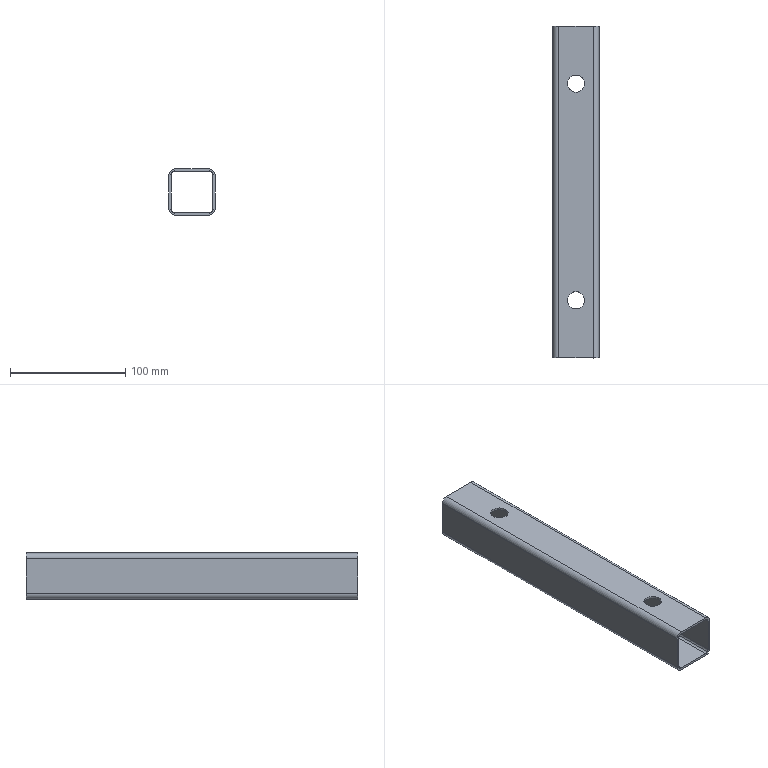Part | NX | features BREP 1 | 1 solid | 44 faces | box 40 x 288 x 40 mm | volume 82180 mm3 | plane 24 | cylinder 20 | commonest cylinder face diameters 6 x8 15 x8 10 x4
STEP:
#1=CARTESIAN_POINT('',(1228.051,-374.5,25.));
#2=VERTEX_POINT('',#1);
#3=CARTESIAN_POINT('',(1228.051,-374.5,27.));
#4=VERTEX_POINT('',#3);
#5=CARTESIAN_POINT('',(1228.051,-374.5,25.));
#6=DIRECTION('',(0.,0.,-1.));
#7=VECTOR('',#6,1000.);
#8=LINE('',#5,#7);
#9=EDGE_CURVE('',#2,#4,#8,.F.);
#10=ORIENTED_EDGE('',*,*,#9,.F.);
#11=CARTESIAN_POINT('',(1213.051,-374.5,25.));
#12=VERTEX_POINT('',#11);
#13=CARTESIAN_POINT('',(1228.051,-374.5,25.));
#14=CARTESIAN_POINT('',(1228.051,-375.305,25.));
#15=CARTESIAN_POINT('',(1227.943,-376.11,25.));
#16=CARTESIAN_POINT('',(1227.727,-376.895,25.));
#17=CARTESIAN_POINT('',(1227.09,-378.389,25.));
#18=CARTESIAN_POINT('',(1226.081,-379.662,25.));
#19=CARTESIAN_POINT('',(1225.494,-380.227,25.));
#20=CARTESIAN_POINT('',(1224.182,-381.185,25.));
#21=CARTESIAN_POINT('',(1222.664,-381.764,25.));
#22=CARTESIAN_POINT('',(1221.871,-381.949,25.));
#23=CARTESIAN_POINT('',(1220.253,-382.102,25.));
#24=CARTESIAN_POINT('',(1218.653,-381.823,25.));
#25=CARTESIAN_POINT('',(1217.876,-381.576,25.));
#26=CARTESIAN_POINT('',(1216.409,-380.881,25.));
#27=CARTESIAN_POINT('',(1215.176,-379.823,25.));
#28=CARTESIAN_POINT('',(1214.634,-379.214,25.));
#29=CARTESIAN_POINT('',(1213.795,-377.964,25.));
#30=CARTESIAN_POINT('',(1213.288,-376.55,25.));
#31=CARTESIAN_POINT('',(1213.13,-375.874,25.));
#32=CARTESIAN_POINT('',(1213.051,-375.187,25.));
#33=CARTESIAN_POINT('',(1213.051,-374.5,25.));
#34=B_SPLINE_CURVE_WITH_KNOTS('',5,(#13,#14,#15,#16,#17,#18,#19,#20,#21,#22,#23,#24,#25,#26,#27,#28,#29,#30,#31,#32,#33),.UNSPECIFIED.,.F.,.F.,(6,3,3,3,3,3,6),(0.,5.692,11.384,17.076,22.768,28.46,33.321),.UNSPECIFIED.);
#35=EDGE_CURVE('',#2,#12,#34,.T.);
#36=ORIENTED_EDGE('',*,*,#35,.T.);
#37=CARTESIAN_POINT('',(1213.051,-374.5,27.));
#38=VERTEX_POINT('',#37);
#39=CARTESIAN_POINT('',(1213.051,-374.5,25.));
#40=DIRECTION('',(0.,0.,-1.));
#41=VECTOR('',#40,1000.);
#42=LINE('',#39,#41);
#43=EDGE_CURVE('',#12,#38,#42,.F.);
#44=ORIENTED_EDGE('',*,*,#43,.T.);
#45=CARTESIAN_POINT('',(1228.051,-374.5,27.));
#46=CARTESIAN_POINT('',(1228.051,-375.305,27.));
#47=CARTESIAN_POINT('',(1227.943,-376.11,27.));
#48=CARTESIAN_POINT('',(1227.727,-376.895,27.));
#49=CARTESIAN_POINT('',(1227.09,-378.389,27.));
#50=CARTESIAN_POINT('',(1226.081,-379.662,27.));
#51=CARTESIAN_POINT('',(1225.494,-380.227,27.));
#52=CARTESIAN_POINT('',(1224.182,-381.185,27.));
#53=CARTESIAN_POINT('',(1222.664,-381.764,27.));
#54=CARTESIAN_POINT('',(1221.871,-381.949,27.));
#55=CARTESIAN_POINT('',(1220.253,-382.102,27.));
#56=CARTESIAN_POINT('',(1218.653,-381.823,27.));
#57=CARTESIAN_POINT('',(1217.876,-381.576,27.));
#58=CARTESIAN_POINT('',(1216.409,-380.881,27.));
#59=CARTESIAN_POINT('',(1215.176,-379.823,27.));
#60=CARTESIAN_POINT('',(1214.634,-379.214,27.));
#61=CARTESIAN_POINT('',(1213.795,-377.964,27.));
#62=CARTESIAN_POINT('',(1213.288,-376.55,27.));
#63=CARTESIAN_POINT('',(1213.13,-375.874,27.));
#64=CARTESIAN_POINT('',(1213.051,-375.187,27.));
#65=CARTESIAN_POINT('',(1213.051,-374.5,27.));
#66=B_SPLINE_CURVE_WITH_KNOTS('',5,(#45,#46,#47,#48,#49,#50,#51,#52,#53,#54,#55,#56,#57,#58,#59,#60,#61,#62,#63,#64,#65),.UNSPECIFIED.,.F.,.F.,(6,3,3,3,3,3,6),(0.,5.692,11.384,17.076,22.768,28.46,33.321),.UNSPECIFIED.);
#67=EDGE_CURVE('',#4,#38,#66,.T.);
#68=ORIENTED_EDGE('',*,*,#67,.F.);
#69=EDGE_LOOP('',(#10,#36,#44,#68));
#70=FACE_BOUND('',#69,.T.);
#71=CARTESIAN_POINT('',(1220.551,-374.5,25.));
#72=DIRECTION('',(0.,0.,-1.));
#73=DIRECTION('',(1.,0.,0.));
#74=AXIS2_PLACEMENT_3D('',#71,#72,#73);
#75=CYLINDRICAL_SURFACE('',#74,7.5);
#76=ADVANCED_FACE('',(#70),#75,.F.);
#77=ORIENTED_EDGE('',*,*,#43,.F.);
#78=CARTESIAN_POINT('',(1213.051,-374.5,25.));
#79=CARTESIAN_POINT('',(1213.051,-373.695,25.));
#80=CARTESIAN_POINT('',(1213.159,-372.89,25.));
#81=CARTESIAN_POINT('',(1213.375,-372.104,25.));
#82=CARTESIAN_POINT('',(1214.013,-370.61,25.));
#83=CARTESIAN_POINT('',(1215.022,-369.337,25.));
#84=CARTESIAN_POINT('',(1215.609,-368.772,25.));
#85=CARTESIAN_POINT('',(1216.921,-367.814,25.));
#86=CARTESIAN_POINT('',(1218.439,-367.235,25.));
#87=CARTESIAN_POINT('',(1219.232,-367.05,25.));
#88=CARTESIAN_POINT('',(1220.849,-366.897,25.));
#89=CARTESIAN_POINT('',(1222.45,-367.176,25.));
#90=CARTESIAN_POINT('',(1223.226,-367.423,25.));
#91=CARTESIAN_POINT('',(1224.694,-368.118,25.));
#92=CARTESIAN_POINT('',(1225.927,-369.176,25.));
#93=CARTESIAN_POINT('',(1226.468,-369.785,25.));
#94=CARTESIAN_POINT('',(1227.308,-371.035,25.));
#95=CARTESIAN_POINT('',(1227.815,-372.449,25.));
#96=CARTESIAN_POINT('',(1227.973,-373.125,25.));
#97=CARTESIAN_POINT('',(1228.051,-373.812,25.));
#98=CARTESIAN_POINT('',(1228.051,-374.5,25.));
#99=B_SPLINE_CURVE_WITH_KNOTS('',5,(#78,#79,#80,#81,#82,#83,#84,#85,#86,#87,#88,#89,#90,#91,#92,#93,#94,#95,#96,#97,#98),.UNSPECIFIED.,.F.,.F.,(6,3,3,3,3,3,6),(0.,5.692,11.384,17.076,22.768,28.46,33.321),.UNSPECIFIED.);
#100=EDGE_CURVE('',#12,#2,#99,.T.);
#101=ORIENTED_EDGE('',*,*,#100,.T.);
#102=ORIENTED_EDGE('',*,*,#9,.T.);
#103=CARTESIAN_POINT('',(1213.051,-374.5,27.));
#104=CARTESIAN_POINT('',(1213.051,-373.695,27.));
#105=CARTESIAN_POINT('',(1213.159,-372.89,27.));
#106=CARTESIAN_POINT('',(1213.375,-372.104,27.));
#107=CARTESIAN_POINT('',(1214.013,-370.61,27.));
#108=CARTESIAN_POINT('',(1215.022,-369.337,27.));
#109=CARTESIAN_POINT('',(1215.609,-368.772,27.));
#110=CARTESIAN_POINT('',(1216.921,-367.814,27.));
#111=CARTESIAN_POINT('',(1218.439,-367.235,27.));
#112=CARTESIAN_POINT('',(1219.232,-367.05,27.));
#113=CARTESIAN_POINT('',(1220.849,-366.897,27.));
#114=CARTESIAN_POINT('',(1222.45,-367.176,27.));
#115=CARTESIAN_POINT('',(1223.226,-367.423,27.));
#116=CARTESIAN_POINT('',(1224.694,-368.118,27.));
#117=CARTESIAN_POINT('',(1225.927,-369.176,27.));
#118=CARTESIAN_POINT('',(1226.468,-369.785,27.));
#119=CARTESIAN_POINT('',(1227.308,-371.035,27.));
#120=CARTESIAN_POINT('',(1227.815,-372.449,27.));
#121=CARTESIAN_POINT('',(1227.973,-373.125,27.));
#122=CARTESIAN_POINT('',(1228.051,-373.812,27.));
#123=CARTESIAN_POINT('',(1228.051,-374.5,27.));
#124=B_SPLINE_CURVE_WITH_KNOTS('',5,(#103,#104,#105,#106,#107,#108,#109,#110,#111,#112,#113,#114,#115,#116,#117,#118,#119,#120,#121,#122,#123),.UNSPECIFIED.,.F.,.F.,(6,3,3,3,3,3,6),(0.,5.692,11.384,17.076,22.768,28.46,33.321),.UNSPECIFIED.);
#125=EDGE_CURVE('',#38,#4,#124,.T.);
#126=ORIENTED_EDGE('',*,*,#125,.F.);
#127=EDGE_LOOP('',(#77,#101,#102,#126));
#128=FACE_BOUND('',#127,.T.);
#129=CARTESIAN_POINT('',(1220.551,-374.5,25.));
#130=DIRECTION('',(0.,0.,-1.));
#131=DIRECTION('',(-1.,0.,0.));
#132=AXIS2_PLACEMENT_3D('',#129,#130,#131);
#133=CYLINDRICAL_SURFACE('',#132,7.5);
#134=ADVANCED_FACE('',(#128),#133,.F.);
#135=CARTESIAN_POINT('',(1213.051,-562.5,25.));
#136=VERTEX_POINT('',#135);
#137=CARTESIAN_POINT('',(1213.051,-562.5,27.));
#138=VERTEX_POINT('',#137);
#139=CARTESIAN_POINT('',(1213.051,-562.5,25.));
#140=DIRECTION('',(0.,0.,1.));
#141=VECTOR('',#140,1000.);
#142=LINE('',#139,#141);
#143=EDGE_CURVE('',#136,#138,#142,.T.);
#144=ORIENTED_EDGE('',*,*,#143,.F.);
#145=CARTESIAN_POINT('',(1228.051,-562.5,25.));
#146=VERTEX_POINT('',#145);
#147=CARTESIAN_POINT('',(1220.551,-562.5,25.));
#148=DIRECTION('',(0.,0.,1.));
#149=DIRECTION('',(1.,0.,0.));
#150=AXIS2_PLACEMENT_3D('',#147,#148,#149);
#151=CIRCLE('',#150,7.5);
#152=EDGE_CURVE('',#146,#136,#151,.T.);
#153=ORIENTED_EDGE('',*,*,#152,.F.);
#154=CARTESIAN_POINT('',(1228.051,-562.5,27.));
#155=VERTEX_POINT('',#154);
#156=CARTESIAN_POINT('',(1228.051,-562.5,25.));
#157=DIRECTION('',(0.,0.,1.));
#158=VECTOR('',#157,1000.);
#159=LINE('',#156,#158);
#160=EDGE_CURVE('',#146,#155,#159,.T.);
#161=ORIENTED_EDGE('',*,*,#160,.T.);
#162=CARTESIAN_POINT('',(1213.051,-562.5,27.));
#163=CARTESIAN_POINT('',(1213.051,-560.53,27.));
#164=CARTESIAN_POINT('',(1214.674,-556.628,27.));
#165=CARTESIAN_POINT('',(1220.551,-554.185,27.));
#166=CARTESIAN_POINT('',(1226.428,-556.628,27.));
#167=CARTESIAN_POINT('',(1228.051,-560.529,27.));
#168=CARTESIAN_POINT('',(1228.051,-562.5,27.));
#169=B_SPLINE_CURVE_WITH_KNOTS('',3,(#162,#163,#164,#165,#166,#167,#168),.UNSPECIFIED.,.F.,.F.,(4,1,1,1,4),(0.,0.25,0.5,0.75,1.),.UNSPECIFIED.);
#170=EDGE_CURVE('',#155,#138,#169,.F.);
#171=ORIENTED_EDGE('',*,*,#170,.T.);
#172=EDGE_LOOP('',(#144,#153,#161,#171));
#173=FACE_BOUND('',#172,.T.);
#174=CARTESIAN_POINT('',(1220.551,-562.5,25.));
#175=DIRECTION('',(0.,0.,1.));
#176=DIRECTION('',(1.,0.,0.));
#177=AXIS2_PLACEMENT_3D('',#174,#175,#176);
#178=CYLINDRICAL_SURFACE('',#177,7.5);
#179=ADVANCED_FACE('',(#173),#178,.F.);
#180=ORIENTED_EDGE('',*,*,#160,.F.);
#181=CARTESIAN_POINT('',(1220.551,-562.5,25.));
#182=DIRECTION('',(0.,0.,1.));
#183=DIRECTION('',(1.,0.,0.));
#184=AXIS2_PLACEMENT_3D('',#181,#182,#183);
#185=CIRCLE('',#184,7.5);
#186=EDGE_CURVE('',#136,#146,#185,.T.);
#187=ORIENTED_EDGE('',*,*,#186,.F.);
#188=ORIENTED_EDGE('',*,*,#143,.T.);
#189=CARTESIAN_POINT('',(1228.051,-562.5,27.));
#190=CARTESIAN_POINT('',(1228.051,-564.469,27.));
#191=CARTESIAN_POINT('',(1226.428,-568.372,27.));
#192=CARTESIAN_POINT('',(1220.551,-570.814,27.));
#193=CARTESIAN_POINT('',(1214.674,-568.371,27.));
#194=CARTESIAN_POINT('',(1213.051,-564.47,27.));
#195=CARTESIAN_POINT('',(1213.051,-562.5,27.));
#196=B_SPLINE_CURVE_WITH_KNOTS('',3,(#189,#190,#191,#192,#193,#194,#195),.UNSPECIFIED.,.F.,.F.,(4,1,1,1,4),(0.,0.25,0.5,0.75,1.),.UNSPECIFIED.);
#197=EDGE_CURVE('',#138,#155,#196,.F.);
#198=ORIENTED_EDGE('',*,*,#197,.T.);
#199=EDGE_LOOP('',(#180,#187,#188,#198));
#200=FACE_BOUND('',#199,.T.);
#201=CARTESIAN_POINT('',(1220.551,-562.5,25.));
#202=DIRECTION('',(0.,0.,1.));
#203=DIRECTION('',(-1.,0.,0.));
#204=AXIS2_PLACEMENT_3D('',#201,#202,#203);
#205=CYLINDRICAL_SURFACE('',#204,7.5);
#206=ADVANCED_FACE('',(#200),#205,.F.);
#207=CARTESIAN_POINT('',(1205.551,-324.5,27.));
#208=VERTEX_POINT('',#207);
#209=CARTESIAN_POINT('',(1205.551,-324.5,25.));
#210=VERTEX_POINT('',#209);
#211=CARTESIAN_POINT('',(1205.551,-324.5,26.));
#212=DIRECTION('',(0.,0.,-1.));
#213=VECTOR('',#212,1000.);
#214=LINE('',#211,#213);
#215=EDGE_CURVE('',#208,#210,#214,.T.);
#216=ORIENTED_EDGE('',*,*,#215,.F.);
#217=CARTESIAN_POINT('',(1235.551,-324.5,27.));
#218=VERTEX_POINT('',#217);
#219=CARTESIAN_POINT('',(1220.551,-324.5,27.));
#220=DIRECTION('',(1.,0.,0.));
#221=VECTOR('',#220,1000.);
#222=LINE('',#219,#221);
#223=EDGE_CURVE('',#208,#218,#222,.T.);
#224=ORIENTED_EDGE('',*,*,#223,.T.);
#225=CARTESIAN_POINT('',(1235.551,-324.5,25.));
#226=VERTEX_POINT('',#225);
#227=CARTESIAN_POINT('',(1235.551,-324.5,26.));
#228=DIRECTION('',(0.,0.,-1.));
#229=VECTOR('',#228,1000.);
#230=LINE('',#227,#229);
#231=EDGE_CURVE('',#218,#226,#230,.T.);
#232=ORIENTED_EDGE('',*,*,#231,.T.);
#233=CARTESIAN_POINT('',(1220.551,-324.5,25.));
#234=DIRECTION('',(1.,0.,0.));
#235=VECTOR('',#234,1000.);
#236=LINE('',#233,#235);
#237=EDGE_CURVE('',#210,#226,#236,.T.);
#238=ORIENTED_EDGE('',*,*,#237,.F.);
#239=EDGE_LOOP('',(#216,#224,#232,#238));
#240=FACE_BOUND('',#239,.T.);
#241=CARTESIAN_POINT('',(1220.551,-324.5,25.));
#242=DIRECTION('',(0.,1.,0.));
#243=DIRECTION('',(1.,0.,0.));
#244=AXIS2_PLACEMENT_3D('',#241,#242,#243);
#245=PLANE('',#244);
#246=ADVANCED_FACE('',(#240),#245,.T.);
#247=CARTESIAN_POINT('',(1240.551,-324.5,30.));
#248=VERTEX_POINT('',#247);
#249=CARTESIAN_POINT('',(1235.551,-324.5,30.));
#250=DIRECTION('',(0.,1.,0.));
#251=DIRECTION('',(1.,0.,0.));
#252=AXIS2_PLACEMENT_3D('',#249,#250,#251);
#253=CIRCLE('',#252,5.);
#254=EDGE_CURVE('',#248,#226,#253,.T.);
#255=ORIENTED_EDGE('',*,*,#254,.T.);
#256=ORIENTED_EDGE('',*,*,#231,.F.);
#257=CARTESIAN_POINT('',(1237.673,-324.5,27.879));
#258=VERTEX_POINT('',#257);
#259=CARTESIAN_POINT('',(1235.551,-324.5,30.));
#260=DIRECTION('',(0.,1.,0.));
#261=DIRECTION('',(1.,0.,0.));
#262=AXIS2_PLACEMENT_3D('',#259,#260,#261);
#263=CIRCLE('',#262,3.);
#264=EDGE_CURVE('',#258,#218,#263,.T.);
#265=ORIENTED_EDGE('',*,*,#264,.F.);
#266=CARTESIAN_POINT('',(1238.551,-324.5,30.));
#267=VERTEX_POINT('',#266);
#268=CARTESIAN_POINT('',(1235.551,-324.5,30.));
#269=DIRECTION('',(0.,1.,0.));
#270=DIRECTION('',(1.,0.,0.));
#271=AXIS2_PLACEMENT_3D('',#268,#269,#270);
#272=CIRCLE('',#271,3.);
#273=EDGE_CURVE('',#267,#258,#272,.T.);
#274=ORIENTED_EDGE('',*,*,#273,.F.);
#275=CARTESIAN_POINT('',(1239.551,-324.5,30.));
#276=DIRECTION('',(1.,0.,0.));
#277=VECTOR('',#276,1000.);
#278=LINE('',#275,#277);
#279=EDGE_CURVE('',#267,#248,#278,.T.);
#280=ORIENTED_EDGE('',*,*,#279,.T.);
#281=EDGE_LOOP('',(#255,#256,#265,#274,#280));
#282=FACE_BOUND('',#281,.T.);
#283=CARTESIAN_POINT('',(1240.551,-324.5,30.));
#284=DIRECTION('',(0.,1.,0.));
#285=DIRECTION('',(-0.3827,0.,-0.9239));
#286=AXIS2_PLACEMENT_3D('',#283,#284,#285);
#287=PLANE('',#286);
#288=ADVANCED_FACE('',(#282),#287,.T.);
#289=ORIENTED_EDGE('',*,*,#67,.T.);
#290=ORIENTED_EDGE('',*,*,#125,.T.);
#291=EDGE_LOOP('',(#289,#290));
#292=FACE_BOUND('',#291,.T.);
#293=ORIENTED_EDGE('',*,*,#170,.F.);
#294=ORIENTED_EDGE('',*,*,#197,.F.);
#295=EDGE_LOOP('',(#293,#294));
#296=FACE_BOUND('',#295,.T.);
#297=CARTESIAN_POINT('',(1205.551,-612.5,27.));
#298=VERTEX_POINT('',#297);
#299=CARTESIAN_POINT('',(1205.551,-468.5,27.));
#300=DIRECTION('',(0.,1.,0.));
#301=VECTOR('',#300,1000.);
#302=LINE('',#299,#301);
#303=EDGE_CURVE('',#298,#208,#302,.T.);
#304=ORIENTED_EDGE('',*,*,#303,.F.);
#305=CARTESIAN_POINT('',(1235.551,-612.5,27.));
#306=VERTEX_POINT('',#305);
#307=CARTESIAN_POINT('',(1220.551,-612.5,27.));
#308=DIRECTION('',(1.,0.,0.));
#309=VECTOR('',#308,1000.);
#310=LINE('',#307,#309);
#311=EDGE_CURVE('',#298,#306,#310,.T.);
#312=ORIENTED_EDGE('',*,*,#311,.T.);
#313=CARTESIAN_POINT('',(1235.551,-468.5,27.));
#314=DIRECTION('',(0.,1.,0.));
#315=VECTOR('',#314,1000.);
#316=LINE('',#313,#315);
#317=EDGE_CURVE('',#306,#218,#316,.T.);
#318=ORIENTED_EDGE('',*,*,#317,.T.);
#319=ORIENTED_EDGE('',*,*,#223,.F.);
#320=EDGE_LOOP('',(#304,#312,#318,#319));
#321=FACE_BOUND('',#320,.T.);
#322=CARTESIAN_POINT('',(1200.551,-612.5,27.));
#323=DIRECTION('',(0.,0.,1.));
#324=DIRECTION('',(1.,0.,0.));
#325=AXIS2_PLACEMENT_3D('',#322,#323,#324);
#326=PLANE('',#325);
#327=ADVANCED_FACE('',(#292,#296,#321),#326,.T.);
#328=ORIENTED_EDGE('',*,*,#100,.F.);
#329=ORIENTED_EDGE('',*,*,#35,.F.);
#330=EDGE_LOOP('',(#328,#329));
#331=FACE_BOUND('',#330,.T.);
#332=ORIENTED_EDGE('',*,*,#186,.T.);
#333=ORIENTED_EDGE('',*,*,#152,.T.);
#334=EDGE_LOOP('',(#332,#333));
#335=FACE_BOUND('',#334,.T.);
#336=ORIENTED_EDGE('',*,*,#237,.T.);
#337=CARTESIAN_POINT('',(1235.551,-612.5,25.));
#338=VERTEX_POINT('',#337);
#339=CARTESIAN_POINT('',(1235.551,-468.5,25.));
#340=DIRECTION('',(0.,1.,0.));
#341=VECTOR('',#340,1000.);
#342=LINE('',#339,#341);
#343=EDGE_CURVE('',#338,#226,#342,.T.);
#344=ORIENTED_EDGE('',*,*,#343,.F.);
#345=CARTESIAN_POINT('',(1205.551,-612.5,25.));
#346=VERTEX_POINT('',#345);
#347=CARTESIAN_POINT('',(1220.551,-612.5,25.));
#348=DIRECTION('',(1.,0.,0.));
#349=VECTOR('',#348,1000.);
#350=LINE('',#347,#349);
#351=EDGE_CURVE('',#346,#338,#350,.T.);
#352=ORIENTED_EDGE('',*,*,#351,.F.);
#353=CARTESIAN_POINT('',(1205.551,-468.5,25.));
#354=DIRECTION('',(0.,1.,0.));
#355=VECTOR('',#354,1000.);
#356=LINE('',#353,#355);
#357=EDGE_CURVE('',#346,#210,#356,.T.);
#358=ORIENTED_EDGE('',*,*,#357,.T.);
#359=EDGE_LOOP('',(#336,#344,#352,#358));
#360=FACE_BOUND('',#359,.T.);
#361=CARTESIAN_POINT('',(1200.551,-612.5,25.));
#362=DIRECTION('',(0.,0.,1.));
#363=DIRECTION('',(1.,0.,0.));
#364=AXIS2_PLACEMENT_3D('',#361,#362,#363);
#365=PLANE('',#364);
#366=ADVANCED_FACE('',(#331,#335,#360),#365,.F.);
#367=CARTESIAN_POINT('',(1202.551,-324.5,30.));
#368=VERTEX_POINT('',#367);
#369=CARTESIAN_POINT('',(1200.551,-324.5,30.));
#370=VERTEX_POINT('',#369);
#371=CARTESIAN_POINT('',(1201.551,-324.5,30.));
#372=DIRECTION('',(-1.,0.,0.));
#373=VECTOR('',#372,1000.);
#374=LINE('',#371,#373);
#375=EDGE_CURVE('',#368,#370,#374,.T.);
#376=ORIENTED_EDGE('',*,*,#375,.F.);
#377=CARTESIAN_POINT('',(1203.43,-324.5,27.879));
#378=VERTEX_POINT('',#377);
#379=CARTESIAN_POINT('',(1205.551,-324.5,30.));
#380=DIRECTION('',(0.,1.,0.));
#381=DIRECTION('',(1.,0.,0.));
#382=AXIS2_PLACEMENT_3D('',#379,#380,#381);
#383=CIRCLE('',#382,3.);
#384=EDGE_CURVE('',#378,#368,#383,.T.);
#385=ORIENTED_EDGE('',*,*,#384,.F.);
#386=CARTESIAN_POINT('',(1205.551,-324.5,30.));
#387=DIRECTION('',(0.,1.,0.));
#388=DIRECTION('',(1.,0.,0.));
#389=AXIS2_PLACEMENT_3D('',#386,#387,#388);
#390=CIRCLE('',#389,3.);
#391=EDGE_CURVE('',#208,#378,#390,.T.);
#392=ORIENTED_EDGE('',*,*,#391,.F.);
#393=ORIENTED_EDGE('',*,*,#215,.T.);
#394=CARTESIAN_POINT('',(1205.551,-324.5,30.));
#395=DIRECTION('',(0.,1.,0.));
#396=DIRECTION('',(1.,0.,0.));
#397=AXIS2_PLACEMENT_3D('',#394,#395,#396);
#398=CIRCLE('',#397,5.);
#399=EDGE_CURVE('',#210,#370,#398,.T.);
#400=ORIENTED_EDGE('',*,*,#399,.T.);
#401=EDGE_LOOP('',(#376,#385,#392,#393,#400));
#402=FACE_BOUND('',#401,.T.);
#403=CARTESIAN_POINT('',(1205.551,-324.5,25.));
#404=DIRECTION('',(0.,1.,0.));
#405=DIRECTION('',(-0.9239,0.,0.3827));
#406=AXIS2_PLACEMENT_3D('',#403,#404,#405);
#407=PLANE('',#406);
#408=ADVANCED_FACE('',(#402),#407,.T.);
#409=CARTESIAN_POINT('',(1240.551,-612.5,30.));
#410=VERTEX_POINT('',#409);
#411=CARTESIAN_POINT('',(1240.551,-468.5,30.));
#412=DIRECTION('',(0.,1.,0.));
#413=VECTOR('',#412,1000.);
#414=LINE('',#411,#413);
#415=EDGE_CURVE('',#410,#248,#414,.T.);
#416=ORIENTED_EDGE('',*,*,#415,.F.);
#417=CARTESIAN_POINT('',(1235.551,-612.5,30.));
#418=DIRECTION('',(0.,1.,0.));
#419=DIRECTION('',(1.,0.,0.));
#420=AXIS2_PLACEMENT_3D('',#417,#418,#419);
#421=CIRCLE('',#420,5.);
#422=EDGE_CURVE('',#410,#338,#421,.T.);
#423=ORIENTED_EDGE('',*,*,#422,.T.);
#424=ORIENTED_EDGE('',*,*,#343,.T.);
#425=ORIENTED_EDGE('',*,*,#254,.F.);
#426=EDGE_LOOP('',(#416,#423,#424,#425));
#427=FACE_BOUND('',#426,.T.);
#428=CARTESIAN_POINT('',(1235.551,-468.5,30.));
#429=DIRECTION('',(0.,1.,0.));
#430=DIRECTION('',(1.,0.,0.));
#431=AXIS2_PLACEMENT_3D('',#428,#429,#430);
#432=CYLINDRICAL_SURFACE('',#431,5.);
#433=ADVANCED_FACE('',(#427),#432,.T.);
#434=ORIENTED_EDGE('',*,*,#264,.T.);
#435=ORIENTED_EDGE('',*,*,#317,.F.);
#436=CARTESIAN_POINT('',(1237.673,-612.5,27.879));
#437=VERTEX_POINT('',#436);
#438=CARTESIAN_POINT('',(1235.551,-612.5,30.));
#439=DIRECTION('',(0.,1.,0.));
#440=DIRECTION('',(1.,0.,0.));
#441=AXIS2_PLACEMENT_3D('',#438,#439,#440);
#442=CIRCLE('',#441,3.);
#443=EDGE_CURVE('',#437,#306,#442,.T.);
#444=ORIENTED_EDGE('',*,*,#443,.F.);
#445=CARTESIAN_POINT('',(1237.673,-468.5,27.879));
#446=DIRECTION('',(0.,1.,0.));
#447=VECTOR('',#446,1000.);
#448=LINE('',#445,#447);
#449=EDGE_CURVE('',#437,#258,#448,.T.);
#450=ORIENTED_EDGE('',*,*,#449,.T.);
#451=EDGE_LOOP('',(#434,#435,#444,#450));
#452=FACE_BOUND('',#451,.T.);
#453=CARTESIAN_POINT('',(1235.551,-468.5,30.));
#454=DIRECTION('',(0.,1.,0.));
#455=DIRECTION('',(0.7071,0.,-0.7071));
#456=AXIS2_PLACEMENT_3D('',#453,#454,#455);
#457=CYLINDRICAL_SURFACE('',#456,3.);
#458=ADVANCED_FACE('',(#452),#457,.F.);
#459=CARTESIAN_POINT('',(1238.551,-612.5,30.));
#460=VERTEX_POINT('',#459);
#461=CARTESIAN_POINT('',(1235.551,-612.5,30.));
#462=DIRECTION('',(0.,1.,0.));
#463=DIRECTION('',(1.,0.,0.));
#464=AXIS2_PLACEMENT_3D('',#461,#462,#463);
#465=CIRCLE('',#464,3.);
#466=EDGE_CURVE('',#460,#437,#465,.T.);
#467=ORIENTED_EDGE('',*,*,#466,.F.);
#468=CARTESIAN_POINT('',(1238.551,-468.5,30.));
#469=DIRECTION('',(0.,1.,0.));
#470=VECTOR('',#469,1000.);
#471=LINE('',#468,#470);
#472=EDGE_CURVE('',#460,#267,#471,.T.);
#473=ORIENTED_EDGE('',*,*,#472,.T.);
#474=ORIENTED_EDGE('',*,*,#273,.T.);
#475=ORIENTED_EDGE('',*,*,#449,.F.);
#476=EDGE_LOOP('',(#467,#473,#474,#475));
#477=FACE_BOUND('',#476,.T.);
#478=CARTESIAN_POINT('',(1235.551,-468.5,30.));
#479=DIRECTION('',(0.,1.,0.));
#480=DIRECTION('',(-0.7071,0.,0.7071));
#481=AXIS2_PLACEMENT_3D('',#478,#479,#480);
#482=CYLINDRICAL_SURFACE('',#481,3.);
#483=ADVANCED_FACE('',(#477),#482,.F.);
#484=CARTESIAN_POINT('',(1240.551,-324.5,60.));
#485=VERTEX_POINT('',#484);
#486=CARTESIAN_POINT('',(1240.551,-324.5,45.));
#487=DIRECTION('',(0.,0.,-1.));
#488=VECTOR('',#487,1000.);
#489=LINE('',#486,#488);
#490=EDGE_CURVE('',#485,#248,#489,.T.);
#491=ORIENTED_EDGE('',*,*,#490,.T.);
#492=ORIENTED_EDGE('',*,*,#279,.F.);
#493=CARTESIAN_POINT('',(1238.551,-324.5,60.));
#494=VERTEX_POINT('',#493);
#495=CARTESIAN_POINT('',(1238.551,-324.5,45.));
#496=DIRECTION('',(0.,0.,-1.));
#497=VECTOR('',#496,1000.);
#498=LINE('',#495,#497);
#499=EDGE_CURVE('',#494,#267,#498,.T.);
#500=ORIENTED_EDGE('',*,*,#499,.F.);
#501=CARTESIAN_POINT('',(1239.551,-324.5,60.));
#502=DIRECTION('',(1.,0.,0.));
#503=VECTOR('',#502,1000.);
#504=LINE('',#501,#503);
#505=EDGE_CURVE('',#494,#485,#504,.T.);
#506=ORIENTED_EDGE('',*,*,#505,.T.);
#507=EDGE_LOOP('',(#491,#492,#500,#506));
#508=FACE_BOUND('',#507,.T.);
#509=CARTESIAN_POINT('',(1240.551,-324.5,45.));
#510=DIRECTION('',(0.,1.,0.));
#511=DIRECTION('',(1.,0.,0.));
#512=AXIS2_PLACEMENT_3D('',#509,#510,#511);
#513=PLANE('',#512);
#514=ADVANCED_FACE('',(#508),#513,.T.);
#515=CARTESIAN_POINT('',(1200.551,-324.5,60.));
#516=VERTEX_POINT('',#515);
#517=CARTESIAN_POINT('',(1200.551,-324.5,45.));
#518=DIRECTION('',(0.,0.,1.));
#519=VECTOR('',#518,1000.);
#520=LINE('',#517,#519);
#521=EDGE_CURVE('',#370,#516,#520,.T.);
#522=ORIENTED_EDGE('',*,*,#521,.T.);
#523=CARTESIAN_POINT('',(1202.551,-324.5,60.));
#524=VERTEX_POINT('',#523);
#525=CARTESIAN_POINT('',(1201.551,-324.5,60.));
#526=DIRECTION('',(-1.,0.,0.));
#527=VECTOR('',#526,1000.);
#528=LINE('',#525,#527);
#529=EDGE_CURVE('',#524,#516,#528,.T.);
#530=ORIENTED_EDGE('',*,*,#529,.F.);
#531=CARTESIAN_POINT('',(1202.551,-324.5,45.));
#532=DIRECTION('',(0.,0.,1.));
#533=VECTOR('',#532,1000.);
#534=LINE('',#531,#533);
#535=EDGE_CURVE('',#368,#524,#534,.T.);
#536=ORIENTED_EDGE('',*,*,#535,.F.);
#537=ORIENTED_EDGE('',*,*,#375,.T.);
#538=EDGE_LOOP('',(#522,#530,#536,#537));
#539=FACE_BOUND('',#538,.T.);
#540=CARTESIAN_POINT('',(1200.551,-324.5,45.));
#541=DIRECTION('',(0.,-1.,0.));
#542=DIRECTION('',(1.,0.,0.));
#543=AXIS2_PLACEMENT_3D('',#540,#541,#542);
#544=PLANE('',#543);
#545=ADVANCED_FACE('',(#539),#544,.F.);
#546=ORIENTED_EDGE('',*,*,#384,.T.);
#547=CARTESIAN_POINT('',(1202.551,-612.5,30.));
#548=VERTEX_POINT('',#547);
#549=CARTESIAN_POINT('',(1202.551,-468.5,30.));
#550=DIRECTION('',(0.,1.,0.));
#551=VECTOR('',#550,1000.);
#552=LINE('',#549,#551);
#553=EDGE_CURVE('',#548,#368,#552,.T.);
#554=ORIENTED_EDGE('',*,*,#553,.F.);
#555=CARTESIAN_POINT('',(1203.43,-612.5,27.879));
#556=VERTEX_POINT('',#555);
#557=CARTESIAN_POINT('',(1205.551,-612.5,30.));
#558=DIRECTION('',(0.,1.,0.));
#559=DIRECTION('',(1.,0.,0.));
#560=AXIS2_PLACEMENT_3D('',#557,#558,#559);
#561=CIRCLE('',#560,3.);
#562=EDGE_CURVE('',#556,#548,#561,.T.);
#563=ORIENTED_EDGE('',*,*,#562,.F.);
#564=CARTESIAN_POINT('',(1203.43,-468.5,27.879));
#565=DIRECTION('',(0.,1.,0.));
#566=VECTOR('',#565,1000.);
#567=LINE('',#564,#566);
#568=EDGE_CURVE('',#556,#378,#567,.T.);
#569=ORIENTED_EDGE('',*,*,#568,.T.);
#570=EDGE_LOOP('',(#546,#554,#563,#569));
#571=FACE_BOUND('',#570,.T.);
#572=CARTESIAN_POINT('',(1205.551,-468.5,30.));
#573=DIRECTION('',(0.,1.,0.));
#574=DIRECTION('',(-0.7071,0.,-0.7071));
#575=AXIS2_PLACEMENT_3D('',#572,#573,#574);
#576=CYLINDRICAL_SURFACE('',#575,3.);
#577=ADVANCED_FACE('',(#571),#576,.F.);
#578=CARTESIAN_POINT('',(1205.551,-612.5,30.));
#579=DIRECTION('',(0.,1.,0.));
#580=DIRECTION('',(1.,0.,0.));
#581=AXIS2_PLACEMENT_3D('',#578,#579,#580);
#582=CIRCLE('',#581,3.);
#583=EDGE_CURVE('',#298,#556,#582,.T.);
#584=ORIENTED_EDGE('',*,*,#583,.F.);
#585=ORIENTED_EDGE('',*,*,#303,.T.);
#586=ORIENTED_EDGE('',*,*,#391,.T.);
#587=ORIENTED_EDGE('',*,*,#568,.F.);
#588=EDGE_LOOP('',(#584,#585,#586,#587));
#589=FACE_BOUND('',#588,.T.);
#590=CARTESIAN_POINT('',(1205.551,-468.5,30.));
#591=DIRECTION('',(0.,1.,0.));
#592=DIRECTION('',(0.7071,0.,0.7071));
#593=AXIS2_PLACEMENT_3D('',#590,#591,#592);
#594=CYLINDRICAL_SURFACE('',#593,3.);
#595=ADVANCED_FACE('',(#589),#594,.F.);
#596=ORIENTED_EDGE('',*,*,#351,.T.);
#597=CARTESIAN_POINT('',(1235.551,-612.5,26.));
#598=DIRECTION('',(0.,0.,-1.));
#599=VECTOR('',#598,1000.);
#600=LINE('',#597,#599);
#601=EDGE_CURVE('',#306,#338,#600,.T.);
#602=ORIENTED_EDGE('',*,*,#601,.F.);
#603=ORIENTED_EDGE('',*,*,#311,.F.);
#604=CARTESIAN_POINT('',(1205.551,-612.5,26.));
#605=DIRECTION('',(0.,0.,-1.));
#606=VECTOR('',#605,1000.);
#607=LINE('',#604,#606);
#608=EDGE_CURVE('',#298,#346,#607,.T.);
#609=ORIENTED_EDGE('',*,*,#608,.T.);
#610=EDGE_LOOP('',(#596,#602,#603,#609));
#611=FACE_BOUND('',#610,.T.);
#612=CARTESIAN_POINT('',(1220.551,-612.5,25.));
#613=DIRECTION('',(0.,1.,0.));
#614=DIRECTION('',(1.,0.,0.));
#615=AXIS2_PLACEMENT_3D('',#612,#613,#614);
#616=PLANE('',#615);
#617=ADVANCED_FACE('',(#611),#616,.F.);
#618=CARTESIAN_POINT('',(1200.551,-612.5,30.));
#619=VERTEX_POINT('',#618);
#620=CARTESIAN_POINT('',(1200.551,-468.5,30.));
#621=DIRECTION('',(0.,1.,0.));
#622=VECTOR('',#621,1000.);
#623=LINE('',#620,#622);
#624=EDGE_CURVE('',#619,#370,#623,.T.);
#625=ORIENTED_EDGE('',*,*,#624,.T.);
#626=ORIENTED_EDGE('',*,*,#399,.F.);
#627=ORIENTED_EDGE('',*,*,#357,.F.);
#628=CARTESIAN_POINT('',(1205.551,-612.5,30.));
#629=DIRECTION('',(0.,1.,0.));
#630=DIRECTION('',(1.,0.,0.));
#631=AXIS2_PLACEMENT_3D('',#628,#629,#630);
#632=CIRCLE('',#631,5.);
#633=EDGE_CURVE('',#346,#619,#632,.T.);
#634=ORIENTED_EDGE('',*,*,#633,.T.);
#635=EDGE_LOOP('',(#625,#626,#627,#634));
#636=FACE_BOUND('',#635,.T.);
#637=CARTESIAN_POINT('',(1205.551,-468.5,30.));
#638=DIRECTION('',(0.,1.,0.));
#639=DIRECTION('',(0.,0.,-1.));
#640=AXIS2_PLACEMENT_3D('',#637,#638,#639);
#641=CYLINDRICAL_SURFACE('',#640,5.);
#642=ADVANCED_FACE('',(#636),#641,.T.);
#643=CARTESIAN_POINT('',(1240.551,-612.5,60.));
#644=VERTEX_POINT('',#643);
#645=CARTESIAN_POINT('',(1240.551,-468.5,60.));
#646=DIRECTION('',(0.,1.,0.));
#647=VECTOR('',#646,1000.);
#648=LINE('',#645,#647);
#649=EDGE_CURVE('',#644,#485,#648,.T.);
#650=ORIENTED_EDGE('',*,*,#649,.F.);
#651=CARTESIAN_POINT('',(1240.551,-612.5,45.));
#652=DIRECTION('',(0.,0.,-1.));
#653=VECTOR('',#652,1000.);
#654=LINE('',#651,#653);
#655=EDGE_CURVE('',#644,#410,#654,.T.);
#656=ORIENTED_EDGE('',*,*,#655,.T.);
#657=ORIENTED_EDGE('',*,*,#415,.T.);
#658=ORIENTED_EDGE('',*,*,#490,.F.);
#659=EDGE_LOOP('',(#650,#656,#657,#658));
#660=FACE_BOUND('',#659,.T.);
#661=CARTESIAN_POINT('',(1240.551,-612.5,65.));
#662=DIRECTION('',(1.,0.,0.));
#663=DIRECTION('',(0.,0.,-1.));
#664=AXIS2_PLACEMENT_3D('',#661,#662,#663);
#665=PLANE('',#664);
#666=ADVANCED_FACE('',(#660),#665,.T.);
#667=CARTESIAN_POINT('',(1239.551,-612.5,30.));
#668=DIRECTION('',(1.,0.,0.));
#669=VECTOR('',#668,1000.);
#670=LINE('',#667,#669);
#671=EDGE_CURVE('',#460,#410,#670,.T.);
#672=ORIENTED_EDGE('',*,*,#671,.F.);
#673=ORIENTED_EDGE('',*,*,#466,.T.);
#674=ORIENTED_EDGE('',*,*,#443,.T.);
#675=ORIENTED_EDGE('',*,*,#601,.T.);
#676=ORIENTED_EDGE('',*,*,#422,.F.);
#677=EDGE_LOOP('',(#672,#673,#674,#675,#676));
#678=FACE_BOUND('',#677,.T.);
#679=CARTESIAN_POINT('',(1240.551,-612.5,30.));
#680=DIRECTION('',(0.,1.,0.));
#681=DIRECTION('',(-0.3827,0.,-0.9239));
#682=AXIS2_PLACEMENT_3D('',#679,#680,#681);
#683=PLANE('',#682);
#684=ADVANCED_FACE('',(#678),#683,.F.);
#685=ORIENTED_EDGE('',*,*,#499,.T.);
#686=ORIENTED_EDGE('',*,*,#472,.F.);
#687=CARTESIAN_POINT('',(1238.551,-612.5,60.));
#688=VERTEX_POINT('',#687);
#689=CARTESIAN_POINT('',(1238.551,-612.5,45.));
#690=DIRECTION('',(0.,0.,-1.));
#691=VECTOR('',#690,1000.);
#692=LINE('',#689,#691);
#693=EDGE_CURVE('',#688,#460,#692,.T.);
#694=ORIENTED_EDGE('',*,*,#693,.F.);
#695=CARTESIAN_POINT('',(1238.551,-468.5,60.));
#696=DIRECTION('',(0.,1.,0.));
#697=VECTOR('',#696,1000.);
#698=LINE('',#695,#697);
#699=EDGE_CURVE('',#688,#494,#698,.T.);
#700=ORIENTED_EDGE('',*,*,#699,.T.);
#701=EDGE_LOOP('',(#685,#686,#694,#700));
#702=FACE_BOUND('',#701,.T.);
#703=CARTESIAN_POINT('',(1238.551,-612.5,65.));
#704=DIRECTION('',(1.,0.,0.));
#705=DIRECTION('',(0.,0.,-1.));
#706=AXIS2_PLACEMENT_3D('',#703,#704,#705);
#707=PLANE('',#706);
#708=ADVANCED_FACE('',(#702),#707,.F.);
#709=CARTESIAN_POINT('',(1235.551,-324.5,65.));
#710=VERTEX_POINT('',#709);
#711=CARTESIAN_POINT('',(1235.551,-324.5,60.));
#712=DIRECTION('',(0.,1.,0.));
#713=DIRECTION('',(1.,0.,0.));
#714=AXIS2_PLACEMENT_3D('',#711,#712,#713);
#715=CIRCLE('',#714,5.);
#716=EDGE_CURVE('',#710,#485,#715,.T.);
#717=ORIENTED_EDGE('',*,*,#716,.T.);
#718=ORIENTED_EDGE('',*,*,#505,.F.);
#719=CARTESIAN_POINT('',(1237.673,-324.5,62.121));
#720=VERTEX_POINT('',#719);
#721=CARTESIAN_POINT('',(1235.551,-324.5,60.));
#722=DIRECTION('',(0.,1.,0.));
#723=DIRECTION('',(1.,0.,0.));
#724=AXIS2_PLACEMENT_3D('',#721,#722,#723);
#725=CIRCLE('',#724,3.);
#726=EDGE_CURVE('',#720,#494,#725,.T.);
#727=ORIENTED_EDGE('',*,*,#726,.F.);
#728=CARTESIAN_POINT('',(1235.551,-324.5,63.));
#729=VERTEX_POINT('',#728);
#730=CARTESIAN_POINT('',(1235.551,-324.5,60.));
#731=DIRECTION('',(0.,1.,0.));
#732=DIRECTION('',(1.,0.,0.));
#733=AXIS2_PLACEMENT_3D('',#730,#731,#732);
#734=CIRCLE('',#733,3.);
#735=EDGE_CURVE('',#729,#720,#734,.T.);
#736=ORIENTED_EDGE('',*,*,#735,.F.);
#737=CARTESIAN_POINT('',(1235.551,-324.5,64.));
#738=DIRECTION('',(0.,0.,-1.));
#739=VECTOR('',#738,1000.);
#740=LINE('',#737,#739);
#741=EDGE_CURVE('',#710,#729,#740,.T.);
#742=ORIENTED_EDGE('',*,*,#741,.F.);
#743=EDGE_LOOP('',(#717,#718,#727,#736,#742));
#744=FACE_BOUND('',#743,.T.);
#745=CARTESIAN_POINT('',(1235.551,-324.5,65.));
#746=DIRECTION('',(0.,1.,0.));
#747=DIRECTION('',(0.9239,0.,-0.3827));
#748=AXIS2_PLACEMENT_3D('',#745,#746,#747);
#749=PLANE('',#748);
#750=ADVANCED_FACE('',(#744),#749,.T.);
#751=CARTESIAN_POINT('',(1205.551,-324.5,65.));
#752=VERTEX_POINT('',#751);
#753=CARTESIAN_POINT('',(1205.551,-324.5,60.));
#754=DIRECTION('',(0.,1.,0.));
#755=DIRECTION('',(1.,0.,0.));
#756=AXIS2_PLACEMENT_3D('',#753,#754,#755);
#757=CIRCLE('',#756,5.);
#758=EDGE_CURVE('',#516,#752,#757,.T.);
#759=ORIENTED_EDGE('',*,*,#758,.T.);
#760=CARTESIAN_POINT('',(1205.551,-324.5,63.));
#761=VERTEX_POINT('',#760);
#762=CARTESIAN_POINT('',(1205.551,-324.5,64.));
#763=DIRECTION('',(0.,0.,-1.));
#764=VECTOR('',#763,1000.);
#765=LINE('',#762,#764);
#766=EDGE_CURVE('',#752,#761,#765,.T.);
#767=ORIENTED_EDGE('',*,*,#766,.T.);
#768=CARTESIAN_POINT('',(1203.43,-324.5,62.121));
#769=VERTEX_POINT('',#768);
#770=CARTESIAN_POINT('',(1205.551,-324.5,60.));
#771=DIRECTION('',(0.,1.,0.));
#772=DIRECTION('',(1.,0.,0.));
#773=AXIS2_PLACEMENT_3D('',#770,#771,#772);
#774=CIRCLE('',#773,3.);
#775=EDGE_CURVE('',#769,#761,#774,.T.);
#776=ORIENTED_EDGE('',*,*,#775,.F.);
#777=CARTESIAN_POINT('',(1205.551,-324.5,60.));
#778=DIRECTION('',(0.,1.,0.));
#779=DIRECTION('',(1.,0.,0.));
#780=AXIS2_PLACEMENT_3D('',#777,#778,#779);
#781=CIRCLE('',#780,3.);
#782=EDGE_CURVE('',#524,#769,#781,.T.);
#783=ORIENTED_EDGE('',*,*,#782,.F.);
#784=ORIENTED_EDGE('',*,*,#529,.T.);
#785=EDGE_LOOP('',(#759,#767,#776,#783,#784));
#786=FACE_BOUND('',#785,.T.);
#787=CARTESIAN_POINT('',(1200.551,-324.5,60.));
#788=DIRECTION('',(0.,1.,0.));
#789=DIRECTION('',(0.3827,0.,0.9239));
#790=AXIS2_PLACEMENT_3D('',#787,#788,#789);
#791=PLANE('',#790);
#792=ADVANCED_FACE('',(#786),#791,.T.);
#793=ORIENTED_EDGE('',*,*,#624,.F.);
#794=CARTESIAN_POINT('',(1200.551,-612.5,60.));
#795=VERTEX_POINT('',#794);
#796=CARTESIAN_POINT('',(1200.551,-612.5,45.));
#797=DIRECTION('',(0.,0.,1.));
#798=VECTOR('',#797,1000.);
#799=LINE('',#796,#798);
#800=EDGE_CURVE('',#619,#795,#799,.T.);
#801=ORIENTED_EDGE('',*,*,#800,.T.);
#802=CARTESIAN_POINT('',(1200.551,-468.5,60.));
#803=DIRECTION('',(0.,1.,0.));
#804=VECTOR('',#803,1000.);
#805=LINE('',#802,#804);
#806=EDGE_CURVE('',#795,#516,#805,.T.);
#807=ORIENTED_EDGE('',*,*,#806,.T.);
#808=ORIENTED_EDGE('',*,*,#521,.F.);
#809=EDGE_LOOP('',(#793,#801,#807,#808));
#810=FACE_BOUND('',#809,.T.);
#811=CARTESIAN_POINT('',(1200.551,-612.5,25.));
#812=DIRECTION('',(-1.,0.,0.));
#813=DIRECTION('',(0.,0.,1.));
#814=AXIS2_PLACEMENT_3D('',#811,#812,#813);
#815=PLANE('',#814);
#816=ADVANCED_FACE('',(#810),#815,.T.);
#817=ORIENTED_EDGE('',*,*,#535,.T.);
#818=CARTESIAN_POINT('',(1202.551,-612.5,60.));
#819=VERTEX_POINT('',#818);
#820=CARTESIAN_POINT('',(1202.551,-468.5,60.));
#821=DIRECTION('',(0.,1.,0.));
#822=VECTOR('',#821,1000.);
#823=LINE('',#820,#822);
#824=EDGE_CURVE('',#819,#524,#823,.T.);
#825=ORIENTED_EDGE('',*,*,#824,.F.);
#826=CARTESIAN_POINT('',(1202.551,-612.5,45.));
#827=DIRECTION('',(0.,0.,1.));
#828=VECTOR('',#827,1000.);
#829=LINE('',#826,#828);
#830=EDGE_CURVE('',#548,#819,#829,.T.);
#831=ORIENTED_EDGE('',*,*,#830,.F.);
#832=ORIENTED_EDGE('',*,*,#553,.T.);
#833=EDGE_LOOP('',(#817,#825,#831,#832));
#834=FACE_BOUND('',#833,.T.);
#835=CARTESIAN_POINT('',(1202.551,-612.5,25.));
#836=DIRECTION('',(-1.,0.,0.));
#837=DIRECTION('',(0.,0.,1.));
#838=AXIS2_PLACEMENT_3D('',#835,#836,#837);
#839=PLANE('',#838);
#840=ADVANCED_FACE('',(#834),#839,.F.);
#841=ORIENTED_EDGE('',*,*,#633,.F.);
#842=ORIENTED_EDGE('',*,*,#608,.F.);
#843=ORIENTED_EDGE('',*,*,#583,.T.);
#844=ORIENTED_EDGE('',*,*,#562,.T.);
#845=CARTESIAN_POINT('',(1201.551,-612.5,30.));
#846=DIRECTION('',(-1.,0.,0.));
#847=VECTOR('',#846,1000.);
#848=LINE('',#845,#847);
#849=EDGE_CURVE('',#548,#619,#848,.T.);
#850=ORIENTED_EDGE('',*,*,#849,.T.);
#851=EDGE_LOOP('',(#841,#842,#843,#844,#850));
#852=FACE_BOUND('',#851,.T.);
#853=CARTESIAN_POINT('',(1205.551,-612.5,25.));
#854=DIRECTION('',(0.,1.,0.));
#855=DIRECTION('',(-0.9239,0.,0.3827));
#856=AXIS2_PLACEMENT_3D('',#853,#854,#855);
#857=PLANE('',#856);
#858=ADVANCED_FACE('',(#852),#857,.F.);
#859=CARTESIAN_POINT('',(1235.551,-612.5,65.));
#860=VERTEX_POINT('',#859);
#861=CARTESIAN_POINT('',(1235.551,-468.5,65.));
#862=DIRECTION('',(0.,1.,0.));
#863=VECTOR('',#862,1000.);
#864=LINE('',#861,#863);
#865=EDGE_CURVE('',#860,#710,#864,.T.);
#866=ORIENTED_EDGE('',*,*,#865,.F.);
#867=CARTESIAN_POINT('',(1235.551,-612.5,60.));
#868=DIRECTION('',(0.,1.,0.));
#869=DIRECTION('',(1.,0.,0.));
#870=AXIS2_PLACEMENT_3D('',#867,#868,#869);
#871=CIRCLE('',#870,5.);
#872=EDGE_CURVE('',#860,#644,#871,.T.);
#873=ORIENTED_EDGE('',*,*,#872,.T.);
#874=ORIENTED_EDGE('',*,*,#649,.T.);
#875=ORIENTED_EDGE('',*,*,#716,.F.);
#876=EDGE_LOOP('',(#866,#873,#874,#875));
#877=FACE_BOUND('',#876,.T.);
#878=CARTESIAN_POINT('',(1235.551,-468.5,60.));
#879=DIRECTION('',(0.,1.,0.));
#880=DIRECTION('',(0.,0.,1.));
#881=AXIS2_PLACEMENT_3D('',#878,#879,#880);
#882=CYLINDRICAL_SURFACE('',#881,5.);
#883=ADVANCED_FACE('',(#877),#882,.T.);
#884=CARTESIAN_POINT('',(1239.551,-612.5,60.));
#885=DIRECTION('',(1.,0.,0.));
#886=VECTOR('',#885,1000.);
#887=LINE('',#884,#886);
#888=EDGE_CURVE('',#688,#644,#887,.T.);
#889=ORIENTED_EDGE('',*,*,#888,.F.);
#890=ORIENTED_EDGE('',*,*,#693,.T.);
#891=ORIENTED_EDGE('',*,*,#671,.T.);
#892=ORIENTED_EDGE('',*,*,#655,.F.);
#893=EDGE_LOOP('',(#889,#890,#891,#892));
#894=FACE_BOUND('',#893,.T.);
#895=CARTESIAN_POINT('',(1240.551,-612.5,45.));
#896=DIRECTION('',(0.,1.,0.));
#897=DIRECTION('',(1.,0.,0.));
#898=AXIS2_PLACEMENT_3D('',#895,#896,#897);
#899=PLANE('',#898);
#900=ADVANCED_FACE('',(#894),#899,.F.);
#901=ORIENTED_EDGE('',*,*,#726,.T.);
#902=ORIENTED_EDGE('',*,*,#699,.F.);
#903=CARTESIAN_POINT('',(1237.673,-612.5,62.121));
#904=VERTEX_POINT('',#903);
#905=CARTESIAN_POINT('',(1235.551,-612.5,60.));
#906=DIRECTION('',(0.,1.,0.));
#907=DIRECTION('',(1.,0.,0.));
#908=AXIS2_PLACEMENT_3D('',#905,#906,#907);
#909=CIRCLE('',#908,3.);
#910=EDGE_CURVE('',#904,#688,#909,.T.);
#911=ORIENTED_EDGE('',*,*,#910,.F.);
#912=CARTESIAN_POINT('',(1237.673,-468.5,62.121));
#913=DIRECTION('',(0.,1.,0.));
#914=VECTOR('',#913,1000.);
#915=LINE('',#912,#914);
#916=EDGE_CURVE('',#904,#720,#915,.T.);
#917=ORIENTED_EDGE('',*,*,#916,.T.);
#918=EDGE_LOOP('',(#901,#902,#911,#917));
#919=FACE_BOUND('',#918,.T.);
#920=CARTESIAN_POINT('',(1235.551,-468.5,60.));
#921=DIRECTION('',(0.,1.,0.));
#922=DIRECTION('',(0.7071,0.,0.7071));
#923=AXIS2_PLACEMENT_3D('',#920,#921,#922);
#924=CYLINDRICAL_SURFACE('',#923,3.);
#925=ADVANCED_FACE('',(#919),#924,.F.);
#926=CARTESIAN_POINT('',(1228.051,-374.5,63.));
#927=VERTEX_POINT('',#926);
#928=CARTESIAN_POINT('',(1228.051,-374.5,65.));
#929=VERTEX_POINT('',#928);
#930=CARTESIAN_POINT('',(1228.051,-374.5,25.));
#931=DIRECTION('',(0.,0.,-1.));
#932=VECTOR('',#931,1000.);
#933=LINE('',#930,#932);
#934=EDGE_CURVE('',#927,#929,#933,.F.);
#935=ORIENTED_EDGE('',*,*,#934,.T.);
#936=CARTESIAN_POINT('',(1213.051,-374.5,65.));
#937=VERTEX_POINT('',#936);
#938=CARTESIAN_POINT('',(1220.551,-374.5,65.));
#939=DIRECTION('',(0.,0.,-1.));
#940=DIRECTION('',(-1.,0.,0.));
#941=AXIS2_PLACEMENT_3D('',#938,#939,#940);
#942=CIRCLE('',#941,7.5);
#943=EDGE_CURVE('',#937,#929,#942,.T.);
#944=ORIENTED_EDGE('',*,*,#943,.F.);
#945=CARTESIAN_POINT('',(1213.051,-374.5,63.));
#946=VERTEX_POINT('',#945);
#947=CARTESIAN_POINT('',(1213.051,-374.5,25.));
#948=DIRECTION('',(0.,0.,-1.));
#949=VECTOR('',#948,1000.);
#950=LINE('',#947,#949);
#951=EDGE_CURVE('',#946,#937,#950,.F.);
#952=ORIENTED_EDGE('',*,*,#951,.F.);
#953=CARTESIAN_POINT('',(1220.551,-374.5,63.));
#954=DIRECTION('',(0.,0.,-1.));
#955=DIRECTION('',(-1.,0.,0.));
#956=AXIS2_PLACEMENT_3D('',#953,#954,#955);
#957=CIRCLE('',#956,7.5);
#958=EDGE_CURVE('',#946,#927,#957,.T.);
#959=ORIENTED_EDGE('',*,*,#958,.T.);
#960=EDGE_LOOP('',(#935,#944,#952,#959));
#961=FACE_BOUND('',#960,.T.);
#962=CARTESIAN_POINT('',(1220.551,-374.5,25.));
#963=DIRECTION('',(0.,0.,-1.));
#964=DIRECTION('',(-1.,0.,0.));
#965=AXIS2_PLACEMENT_3D('',#962,#963,#964);
#966=CYLINDRICAL_SURFACE('',#965,7.5);
#967=ADVANCED_FACE('',(#961),#966,.F.);
#968=ORIENTED_EDGE('',*,*,#951,.T.);
#969=CARTESIAN_POINT('',(1220.551,-374.5,65.));
#970=DIRECTION('',(0.,0.,-1.));
#971=DIRECTION('',(-1.,0.,0.));
#972=AXIS2_PLACEMENT_3D('',#969,#970,#971);
#973=CIRCLE('',#972,7.5);
#974=EDGE_CURVE('',#929,#937,#973,.T.);
#975=ORIENTED_EDGE('',*,*,#974,.F.);
#976=ORIENTED_EDGE('',*,*,#934,.F.);
#977=CARTESIAN_POINT('',(1220.551,-374.5,63.));
#978=DIRECTION('',(0.,0.,-1.));
#979=DIRECTION('',(-1.,0.,0.));
#980=AXIS2_PLACEMENT_3D('',#977,#978,#979);
#981=CIRCLE('',#980,7.5);
#982=EDGE_CURVE('',#927,#946,#981,.T.);
#983=ORIENTED_EDGE('',*,*,#982,.T.);
#984=EDGE_LOOP('',(#968,#975,#976,#983));
#985=FACE_BOUND('',#984,.T.);
#986=CARTESIAN_POINT('',(1220.551,-374.5,25.));
#987=DIRECTION('',(0.,0.,-1.));
#988=DIRECTION('',(1.,0.,0.));
#989=AXIS2_PLACEMENT_3D('',#986,#987,#988);
#990=CYLINDRICAL_SURFACE('',#989,7.5);
#991=ADVANCED_FACE('',(#985),#990,.F.);
#992=CARTESIAN_POINT('',(1213.051,-562.5,63.));
#993=VERTEX_POINT('',#992);
#994=CARTESIAN_POINT('',(1213.051,-562.5,65.));
#995=VERTEX_POINT('',#994);
#996=CARTESIAN_POINT('',(1213.051,-562.5,25.));
#997=DIRECTION('',(0.,0.,1.));
#998=VECTOR('',#997,1000.);
#999=LINE('',#996,#998);
#1000=EDGE_CURVE('',#993,#995,#999,.T.);
#1001=ORIENTED_EDGE('',*,*,#1000,.T.);
#1002=CARTESIAN_POINT('',(1228.051,-562.5,65.));
#1003=VERTEX_POINT('',#1002);
#1004=CARTESIAN_POINT('',(1220.551,-562.5,65.));
#1005=DIRECTION('',(0.,0.,-1.));
#1006=DIRECTION('',(-1.,0.,0.));
#1007=AXIS2_PLACEMENT_3D('',#1004,#1005,#1006);
#1008=CIRCLE('',#1007,7.5);
#1009=EDGE_CURVE('',#1003,#995,#1008,.T.);
#1010=ORIENTED_EDGE('',*,*,#1009,.F.);
#1011=CARTESIAN_POINT('',(1228.051,-562.5,63.));
#1012=VERTEX_POINT('',#1011);
#1013=CARTESIAN_POINT('',(1228.051,-562.5,25.));
#1014=DIRECTION('',(0.,0.,1.));
#1015=VECTOR('',#1014,1000.);
#1016=LINE('',#1013,#1015);
#1017=EDGE_CURVE('',#1012,#1003,#1016,.T.);
#1018=ORIENTED_EDGE('',*,*,#1017,.F.);
#1019=CARTESIAN_POINT('',(1213.051,-562.5,63.));
#1020=CARTESIAN_POINT('',(1213.051,-564.469,63.));
#1021=CARTESIAN_POINT('',(1214.674,-568.372,63.));
#1022=CARTESIAN_POINT('',(1220.551,-570.814,63.));
#1023=CARTESIAN_POINT('',(1226.428,-568.371,63.));
#1024=CARTESIAN_POINT('',(1228.051,-564.47,63.));
#1025=CARTESIAN_POINT('',(1228.051,-562.5,63.));
#1026=B_SPLINE_CURVE_WITH_KNOTS('',3,(#1019,#1020,#1021,#1022,#1023,#1024,#1025),.UNSPECIFIED.,.F.,.F.,(4,1,1,1,4),(0.,0.25,0.5,0.75,1.),.UNSPECIFIED.);
#1027=EDGE_CURVE('',#1012,#993,#1026,.F.);
#1028=ORIENTED_EDGE('',*,*,#1027,.T.);
#1029=EDGE_LOOP('',(#1001,#1010,#1018,#1028));
#1030=FACE_BOUND('',#1029,.T.);
#1031=CARTESIAN_POINT('',(1220.551,-562.5,25.));
#1032=DIRECTION('',(0.,0.,1.));
#1033=DIRECTION('',(-1.,0.,0.));
#1034=AXIS2_PLACEMENT_3D('',#1031,#1032,#1033);
#1035=CYLINDRICAL_SURFACE('',#1034,7.5);
#1036=ADVANCED_FACE('',(#1030),#1035,.F.);
#1037=ORIENTED_EDGE('',*,*,#1017,.T.);
#1038=CARTESIAN_POINT('',(1220.551,-562.5,65.));
#1039=DIRECTION('',(0.,0.,-1.));
#1040=DIRECTION('',(-1.,0.,0.));
#1041=AXIS2_PLACEMENT_3D('',#1038,#1039,#1040);
#1042=CIRCLE('',#1041,7.5);
#1043=EDGE_CURVE('',#995,#1003,#1042,.T.);
#1044=ORIENTED_EDGE('',*,*,#1043,.F.);
#1045=ORIENTED_EDGE('',*,*,#1000,.F.);
#1046=CARTESIAN_POINT('',(1228.051,-562.5,63.));
#1047=CARTESIAN_POINT('',(1228.051,-560.53,63.));
#1048=CARTESIAN_POINT('',(1226.428,-556.628,63.));
#1049=CARTESIAN_POINT('',(1220.551,-554.185,63.));
#1050=CARTESIAN_POINT('',(1214.674,-556.628,63.));
#1051=CARTESIAN_POINT('',(1213.051,-560.529,63.));
#1052=CARTESIAN_POINT('',(1213.051,-562.5,63.));
#1053=B_SPLINE_CURVE_WITH_KNOTS('',3,(#1046,#1047,#1048,#1049,#1050,#1051,#1052),.UNSPECIFIED.,.F.,.F.,(4,1,1,1,4),(0.,0.25,0.5,0.75,1.),.UNSPECIFIED.);
#1054=EDGE_CURVE('',#993,#1012,#1053,.F.);
#1055=ORIENTED_EDGE('',*,*,#1054,.T.);
#1056=EDGE_LOOP('',(#1037,#1044,#1045,#1055));
#1057=FACE_BOUND('',#1056,.T.);
#1058=CARTESIAN_POINT('',(1220.551,-562.5,25.));
#1059=DIRECTION('',(0.,0.,1.));
#1060=DIRECTION('',(1.,0.,0.));
#1061=AXIS2_PLACEMENT_3D('',#1058,#1059,#1060);
#1062=CYLINDRICAL_SURFACE('',#1061,7.5);
#1063=ADVANCED_FACE('',(#1057),#1062,.F.);
#1064=CARTESIAN_POINT('',(1235.551,-612.5,63.));
#1065=VERTEX_POINT('',#1064);
#1066=CARTESIAN_POINT('',(1235.551,-612.5,60.));
#1067=DIRECTION('',(0.,1.,0.));
#1068=DIRECTION('',(1.,0.,0.));
#1069=AXIS2_PLACEMENT_3D('',#1066,#1067,#1068);
#1070=CIRCLE('',#1069,3.);
#1071=EDGE_CURVE('',#1065,#904,#1070,.T.);
#1072=ORIENTED_EDGE('',*,*,#1071,.F.);
#1073=CARTESIAN_POINT('',(1235.551,-468.5,63.));
#1074=DIRECTION('',(0.,1.,0.));
#1075=VECTOR('',#1074,1000.);
#1076=LINE('',#1073,#1075);
#1077=EDGE_CURVE('',#1065,#729,#1076,.T.);
#1078=ORIENTED_EDGE('',*,*,#1077,.T.);
#1079=ORIENTED_EDGE('',*,*,#735,.T.);
#1080=ORIENTED_EDGE('',*,*,#916,.F.);
#1081=EDGE_LOOP('',(#1072,#1078,#1079,#1080));
#1082=FACE_BOUND('',#1081,.T.);
#1083=CARTESIAN_POINT('',(1235.551,-468.5,60.));
#1084=DIRECTION('',(0.,1.,0.));
#1085=DIRECTION('',(-0.7071,0.,-0.7071));
#1086=AXIS2_PLACEMENT_3D('',#1083,#1084,#1085);
#1087=CYLINDRICAL_SURFACE('',#1086,3.);
#1088=ADVANCED_FACE('',(#1082),#1087,.F.);
#1089=CARTESIAN_POINT('',(1220.551,-324.5,65.));
#1090=DIRECTION('',(1.,0.,0.));
#1091=VECTOR('',#1090,1000.);
#1092=LINE('',#1089,#1091);
#1093=EDGE_CURVE('',#752,#710,#1092,.T.);
#1094=ORIENTED_EDGE('',*,*,#1093,.T.);
#1095=ORIENTED_EDGE('',*,*,#741,.T.);
#1096=CARTESIAN_POINT('',(1220.551,-324.5,63.));
#1097=DIRECTION('',(1.,0.,0.));
#1098=VECTOR('',#1097,1000.);
#1099=LINE('',#1096,#1098);
#1100=EDGE_CURVE('',#761,#729,#1099,.T.);
#1101=ORIENTED_EDGE('',*,*,#1100,.F.);
#1102=ORIENTED_EDGE('',*,*,#766,.F.);
#1103=EDGE_LOOP('',(#1094,#1095,#1101,#1102));
#1104=FACE_BOUND('',#1103,.T.);
#1105=CARTESIAN_POINT('',(1220.551,-324.5,65.));
#1106=DIRECTION('',(0.,-1.,0.));
#1107=DIRECTION('',(1.,0.,0.));
#1108=AXIS2_PLACEMENT_3D('',#1105,#1106,#1107);
#1109=PLANE('',#1108);
#1110=ADVANCED_FACE('',(#1104),#1109,.F.);
#1111=ORIENTED_EDGE('',*,*,#806,.F.);
#1112=CARTESIAN_POINT('',(1205.551,-612.5,65.));
#1113=VERTEX_POINT('',#1112);
#1114=CARTESIAN_POINT('',(1205.551,-612.5,60.));
#1115=DIRECTION('',(0.,1.,0.));
#1116=DIRECTION('',(1.,0.,0.));
#1117=AXIS2_PLACEMENT_3D('',#1114,#1115,#1116);
#1118=CIRCLE('',#1117,5.);
#1119=EDGE_CURVE('',#795,#1113,#1118,.T.);
#1120=ORIENTED_EDGE('',*,*,#1119,.T.);
#1121=CARTESIAN_POINT('',(1205.551,-468.5,65.));
#1122=DIRECTION('',(0.,1.,0.));
#1123=VECTOR('',#1122,1000.);
#1124=LINE('',#1121,#1123);
#1125=EDGE_CURVE('',#1113,#752,#1124,.T.);
#1126=ORIENTED_EDGE('',*,*,#1125,.T.);
#1127=ORIENTED_EDGE('',*,*,#758,.F.);
#1128=EDGE_LOOP('',(#1111,#1120,#1126,#1127));
#1129=FACE_BOUND('',#1128,.T.);
#1130=CARTESIAN_POINT('',(1205.551,-468.5,60.));
#1131=DIRECTION('',(0.,1.,0.));
#1132=DIRECTION('',(-1.,0.,0.));
#1133=AXIS2_PLACEMENT_3D('',#1130,#1131,#1132);
#1134=CYLINDRICAL_SURFACE('',#1133,5.);
#1135=ADVANCED_FACE('',(#1129),#1134,.T.);
#1136=ORIENTED_EDGE('',*,*,#775,.T.);
#1137=CARTESIAN_POINT('',(1205.551,-612.5,63.));
#1138=VERTEX_POINT('',#1137);
#1139=CARTESIAN_POINT('',(1205.551,-468.5,63.));
#1140=DIRECTION('',(0.,1.,0.));
#1141=VECTOR('',#1140,1000.);
#1142=LINE('',#1139,#1141);
#1143=EDGE_CURVE('',#1138,#761,#1142,.T.);
#1144=ORIENTED_EDGE('',*,*,#1143,.F.);
#1145=CARTESIAN_POINT('',(1203.43,-612.5,62.121));
#1146=VERTEX_POINT('',#1145);
#1147=CARTESIAN_POINT('',(1205.551,-612.5,60.));
#1148=DIRECTION('',(0.,1.,0.));
#1149=DIRECTION('',(1.,0.,0.));
#1150=AXIS2_PLACEMENT_3D('',#1147,#1148,#1149);
#1151=CIRCLE('',#1150,3.);
#1152=EDGE_CURVE('',#1146,#1138,#1151,.T.);
#1153=ORIENTED_EDGE('',*,*,#1152,.F.);
#1154=CARTESIAN_POINT('',(1203.43,-468.5,62.121));
#1155=DIRECTION('',(0.,1.,0.));
#1156=VECTOR('',#1155,1000.);
#1157=LINE('',#1154,#1156);
#1158=EDGE_CURVE('',#1146,#769,#1157,.T.);
#1159=ORIENTED_EDGE('',*,*,#1158,.T.);
#1160=EDGE_LOOP('',(#1136,#1144,#1153,#1159));
#1161=FACE_BOUND('',#1160,.T.);
#1162=CARTESIAN_POINT('',(1205.551,-468.5,60.));
#1163=DIRECTION('',(0.,1.,0.));
#1164=DIRECTION('',(-0.7071,0.,0.7071));
#1165=AXIS2_PLACEMENT_3D('',#1162,#1163,#1164);
#1166=CYLINDRICAL_SURFACE('',#1165,3.);
#1167=ADVANCED_FACE('',(#1161),#1166,.F.);
#1168=CARTESIAN_POINT('',(1205.551,-612.5,60.));
#1169=DIRECTION('',(0.,1.,0.));
#1170=DIRECTION('',(1.,0.,0.));
#1171=AXIS2_PLACEMENT_3D('',#1168,#1169,#1170);
#1172=CIRCLE('',#1171,3.);
#1173=EDGE_CURVE('',#819,#1146,#1172,.T.);
#1174=ORIENTED_EDGE('',*,*,#1173,.F.);
#1175=ORIENTED_EDGE('',*,*,#824,.T.);
#1176=ORIENTED_EDGE('',*,*,#782,.T.);
#1177=ORIENTED_EDGE('',*,*,#1158,.F.);
#1178=EDGE_LOOP('',(#1174,#1175,#1176,#1177));
#1179=FACE_BOUND('',#1178,.T.);
#1180=CARTESIAN_POINT('',(1205.551,-468.5,60.));
#1181=DIRECTION('',(0.,1.,0.));
#1182=DIRECTION('',(0.7071,0.,-0.7071));
#1183=AXIS2_PLACEMENT_3D('',#1180,#1181,#1182);
#1184=CYLINDRICAL_SURFACE('',#1183,3.);
#1185=ADVANCED_FACE('',(#1179),#1184,.F.);
#1186=ORIENTED_EDGE('',*,*,#849,.F.);
#1187=ORIENTED_EDGE('',*,*,#830,.T.);
#1188=CARTESIAN_POINT('',(1201.551,-612.5,60.));
#1189=DIRECTION('',(-1.,0.,0.));
#1190=VECTOR('',#1189,1000.);
#1191=LINE('',#1188,#1190);
#1192=EDGE_CURVE('',#819,#795,#1191,.T.);
#1193=ORIENTED_EDGE('',*,*,#1192,.T.);
#1194=ORIENTED_EDGE('',*,*,#800,.F.);
#1195=EDGE_LOOP('',(#1186,#1187,#1193,#1194));
#1196=FACE_BOUND('',#1195,.T.);
#1197=CARTESIAN_POINT('',(1200.551,-612.5,45.));
#1198=DIRECTION('',(0.,-1.,0.));
#1199=DIRECTION('',(1.,0.,0.));
#1200=AXIS2_PLACEMENT_3D('',#1197,#1198,#1199);
#1201=PLANE('',#1200);
#1202=ADVANCED_FACE('',(#1196),#1201,.T.);
#1203=ORIENTED_EDGE('',*,*,#943,.T.);
#1204=ORIENTED_EDGE('',*,*,#974,.T.);
#1205=EDGE_LOOP('',(#1203,#1204));
#1206=FACE_BOUND('',#1205,.T.);
#1207=ORIENTED_EDGE('',*,*,#1009,.T.);
#1208=ORIENTED_EDGE('',*,*,#1043,.T.);
#1209=EDGE_LOOP('',(#1207,#1208));
#1210=FACE_BOUND('',#1209,.T.);
#1211=CARTESIAN_POINT('',(1220.551,-612.5,65.));
#1212=DIRECTION('',(1.,0.,0.));
#1213=VECTOR('',#1212,1000.);
#1214=LINE('',#1211,#1213);
#1215=EDGE_CURVE('',#1113,#860,#1214,.T.);
#1216=ORIENTED_EDGE('',*,*,#1215,.T.);
#1217=ORIENTED_EDGE('',*,*,#865,.T.);
#1218=ORIENTED_EDGE('',*,*,#1093,.F.);
#1219=ORIENTED_EDGE('',*,*,#1125,.F.);
#1220=EDGE_LOOP('',(#1216,#1217,#1218,#1219));
#1221=FACE_BOUND('',#1220,.T.);
#1222=CARTESIAN_POINT('',(1240.551,-612.5,65.));
#1223=DIRECTION('',(0.,0.,-1.));
#1224=DIRECTION('',(-1.,0.,0.));
#1225=AXIS2_PLACEMENT_3D('',#1222,#1223,#1224);
#1226=PLANE('',#1225);
#1227=ADVANCED_FACE('',(#1206,#1210,#1221),#1226,.F.);
#1228=CARTESIAN_POINT('',(1235.551,-612.5,64.));
#1229=DIRECTION('',(0.,0.,-1.));
#1230=VECTOR('',#1229,1000.);
#1231=LINE('',#1228,#1230);
#1232=EDGE_CURVE('',#860,#1065,#1231,.T.);
#1233=ORIENTED_EDGE('',*,*,#1232,.T.);
#1234=ORIENTED_EDGE('',*,*,#1071,.T.);
#1235=ORIENTED_EDGE('',*,*,#910,.T.);
#1236=ORIENTED_EDGE('',*,*,#888,.T.);
#1237=ORIENTED_EDGE('',*,*,#872,.F.);
#1238=EDGE_LOOP('',(#1233,#1234,#1235,#1236,#1237));
#1239=FACE_BOUND('',#1238,.T.);
#1240=CARTESIAN_POINT('',(1235.551,-612.5,65.));
#1241=DIRECTION('',(0.,1.,0.));
#1242=DIRECTION('',(0.9239,0.,-0.3827));
#1243=AXIS2_PLACEMENT_3D('',#1240,#1241,#1242);
#1244=PLANE('',#1243);
#1245=ADVANCED_FACE('',(#1239),#1244,.F.);
#1246=ORIENTED_EDGE('',*,*,#982,.F.);
#1247=ORIENTED_EDGE('',*,*,#958,.F.);
#1248=EDGE_LOOP('',(#1246,#1247));
#1249=FACE_BOUND('',#1248,.T.);
#1250=ORIENTED_EDGE('',*,*,#1054,.F.);
#1251=ORIENTED_EDGE('',*,*,#1027,.F.);
#1252=EDGE_LOOP('',(#1250,#1251));
#1253=FACE_BOUND('',#1252,.T.);
#1254=ORIENTED_EDGE('',*,*,#1143,.T.);
#1255=ORIENTED_EDGE('',*,*,#1100,.T.);
#1256=ORIENTED_EDGE('',*,*,#1077,.F.);
#1257=CARTESIAN_POINT('',(1220.551,-612.5,63.));
#1258=DIRECTION('',(1.,0.,0.));
#1259=VECTOR('',#1258,1000.);
#1260=LINE('',#1257,#1259);
#1261=EDGE_CURVE('',#1138,#1065,#1260,.T.);
#1262=ORIENTED_EDGE('',*,*,#1261,.F.);
#1263=EDGE_LOOP('',(#1254,#1255,#1256,#1262));
#1264=FACE_BOUND('',#1263,.T.);
#1265=CARTESIAN_POINT('',(1240.551,-612.5,63.));
#1266=DIRECTION('',(0.,0.,-1.));
#1267=DIRECTION('',(-1.,0.,0.));
#1268=AXIS2_PLACEMENT_3D('',#1265,#1266,#1267);
#1269=PLANE('',#1268);
#1270=ADVANCED_FACE('',(#1249,#1253,#1264),#1269,.T.);
#1271=ORIENTED_EDGE('',*,*,#1192,.F.);
#1272=ORIENTED_EDGE('',*,*,#1173,.T.);
#1273=ORIENTED_EDGE('',*,*,#1152,.T.);
#1274=CARTESIAN_POINT('',(1205.551,-612.5,64.));
#1275=DIRECTION('',(0.,0.,-1.));
#1276=VECTOR('',#1275,1000.);
#1277=LINE('',#1274,#1276);
#1278=EDGE_CURVE('',#1113,#1138,#1277,.T.);
#1279=ORIENTED_EDGE('',*,*,#1278,.F.);
#1280=ORIENTED_EDGE('',*,*,#1119,.F.);
#1281=EDGE_LOOP('',(#1271,#1272,#1273,#1279,#1280));
#1282=FACE_BOUND('',#1281,.T.);
#1283=CARTESIAN_POINT('',(1200.551,-612.5,60.));
#1284=DIRECTION('',(0.,1.,0.));
#1285=DIRECTION('',(0.3827,0.,0.9239));
#1286=AXIS2_PLACEMENT_3D('',#1283,#1284,#1285);
#1287=PLANE('',#1286);
#1288=ADVANCED_FACE('',(#1282),#1287,.F.);
#1289=ORIENTED_EDGE('',*,*,#1278,.T.);
#1290=ORIENTED_EDGE('',*,*,#1261,.T.);
#1291=ORIENTED_EDGE('',*,*,#1232,.F.);
#1292=ORIENTED_EDGE('',*,*,#1215,.F.);
#1293=EDGE_LOOP('',(#1289,#1290,#1291,#1292));
#1294=FACE_BOUND('',#1293,.T.);
#1295=CARTESIAN_POINT('',(1220.551,-612.5,65.));
#1296=DIRECTION('',(0.,-1.,0.));
#1297=DIRECTION('',(1.,0.,0.));
#1298=AXIS2_PLACEMENT_3D('',#1295,#1296,#1297);
#1299=PLANE('',#1298);
#1300=ADVANCED_FACE('',(#1294),#1299,.T.);
#1301=CLOSED_SHELL('',(#76,#134,#179,#206,#246,#288,#327,#366,#408,#433,#458,#483,#514,#545,#577,#595,#617,#642,#666,#684,#708,#750,#792,#816,#840,#858,#883,#900,#925,#967,#991,#1036,#1063,#1088,#1110,#1135,#1167,#1185,#1202,#1227,#1245,#1270,#1288,#1300));
#1302=MANIFOLD_SOLID_BREP('',#1301);
#1303=(LENGTH_UNIT()NAMED_UNIT(*)SI_UNIT(.MILLI.,.METRE.));
#1304=UNCERTAINTY_MEASURE_WITH_UNIT(LENGTH_MEASURE(0.0508),#1303,'','');
#1305=(NAMED_UNIT(*)PLANE_ANGLE_UNIT()SI_UNIT($,.RADIAN.));
#1306=(NAMED_UNIT(*)SI_UNIT($,.STERADIAN.)SOLID_ANGLE_UNIT());
#1307=(GEOMETRIC_REPRESENTATION_CONTEXT(3)GLOBAL_UNCERTAINTY_ASSIGNED_CONTEXT((#1304))GLOBAL_UNIT_ASSIGNED_CONTEXT((#1303,#1305,#1306))REPRESENTATION_CONTEXT('',''));
#1308=ADVANCED_BREP_SHAPE_REPRESENTATION('',(#1302),#1307);